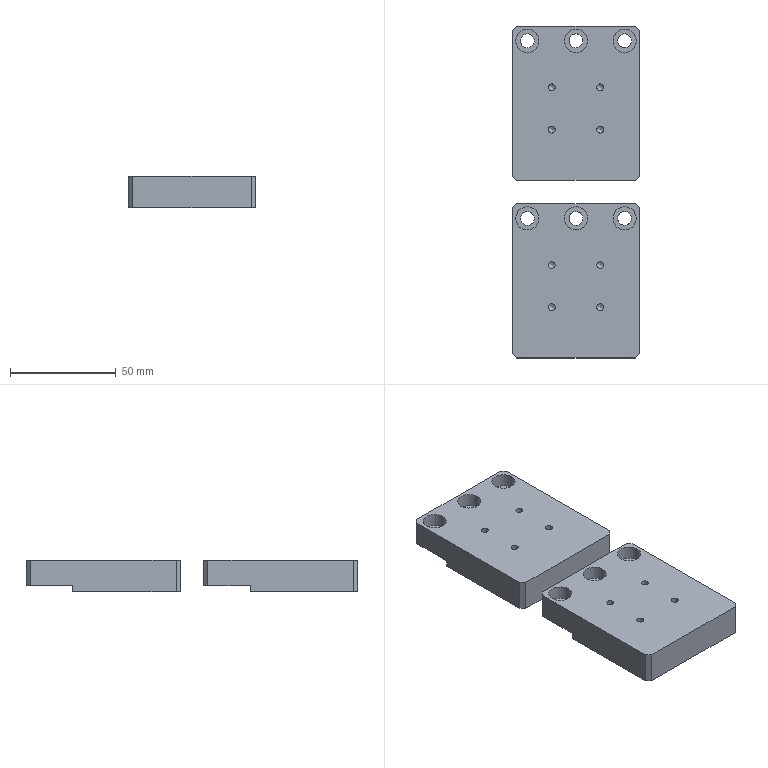CAM job | NX | 3-axis milling, drilling | part box 60 x 157 x 15 mm | stock box 65 x 162 x 20 mm
Tools:
number,name,description,diameter,corner_radius,flute_length,length,flutes
6,D6,平底铣刀-粗,6.0,0.0,25.0,75.0,2
9,D10,平底铣刀-粗,10.0,0.0,35.0,75.0,2
7,D6-J,平底铣刀-精,6.0,0.0,25.0,75.0,2
10,D10-J,平底铣刀-精,10.0,0.0,35.0,75.0,2
1,D80R0.8飞刀,圆鼻刀-粗,80.0,0.8,50.0,75.0,2
1,D80R0.8飞刀-J,圆鼻刀-精,80.0,0.8,50.0,75.0,2
2,D6倒角刀,倒角刀,6.0,0.0,3.0,25.0,2
21,M4X0.7,丝锥,3.3,0.0,35.0,50.0,2
17,ZT6.6,钻头,6.6,0.0,35.0,50.0,2
13,钻头3.3,Twist Drill 3.3 mm,3.3,0.0,35.0,35.008,2
Operations:
program,operation,operation_type,tool,method,geometry_group,spindle_rpm,surface_speed,feed_per_tooth,feed_cut,feed_plunge,cut_length_mm,path_length_mm,cut_time_min,machine_time_min
B,底壁铣飞面一刀开粗_COPY,VolumeBased25DMillingOperation,D80R0.8飞刀,分层开粗-切深K-步距G,W-B,2800.0,703.696,0.5357,3000.0,100.0,2386.746,4674.966,0.7956,1.024
B,底壁铣飞面一刀精光_COPY,VolumeBased25DMillingOperation,D80R0.8飞刀-J,侧刃精光-切深K-步距G,W-B,4000.0,1005.28,0.125,1000.0,100.0,264.998,300.998,0.265,0.2686
B,底壁铣分层开粗-中_COPY,VolumeBased25DMillingOperation,D10,分层开粗-切深K-步距G,W-B,8000.0,251.32,0.25,4000.0,100.0,3038.93,3339.684,0.7597,0.7898
B,铣倒角_2,PlanarMilling,D6倒角刀,METHOD,W-B,8000.0,150.796,0.075,1200.0,100.0,122.676,588.061,0.1022,0.1488
B,C0.3平面去毛刺6X45L__COPY,SurfaceContour,D6倒角刀,爬面_倒角-切深0-步距G,W-B,8000.0,150.796,0.0938,1500.0,90.0,779.275,1448.738,0.5211,0.588
B,底壁铣精光底面-中_COPY,VolumeBased25DMillingOperation,D10-J,精光步距切深关,W-B,8000.0,251.32,0.0625,1000.0,100.0,742.944,931.194,0.7429,0.7618
B,底壁铣精光侧面-中-选底面_COPY,VolumeBased25DMillingOperation,D10-J,侧刃精光-切深K-步距G,W-B,8000.0,251.32,0.0625,1000.0,100.0,157.364,335.31,0.1574,0.1752
A,顶面,FaceMilling,D80R0.8飞刀,侧刃精光-切深K-步距G,W-A,4000.0,1005.31,0.125,1000.0,100.0,534.667,570.667,0.5347,0.5383
A,外形粗_2,VolumeBased25DMillingOperation,D10,METHOD,W-A,8000.0,251.327,0.3125,5000.0,80.0,12324.077,12515.177,2.465,2.484
A,打点-深0.8,Operation,D6倒角刀,NONE,W-A,8000.0,150.796,0.0312,500.0,90.0,25.2,416.7,0.0504,0.0895
A,沉头孔-钻孔0段,Operation,ZT6.6,NONE,W-A,1200.0,24.881,0.0625,150.0,90.0,101.897,424.887,0.6793,0.7116
A,盲锥孔-M4螺纹底孔,Operation,钻头3.3,NONE,W-A,3000.0,31.102,0.02,120.0,90.0,112.0,461.151,0.9333,0.9682
A,铣孔开粗D6_1,CylinderMilling,D6,NONE,W-A,8000.0,150.796,0.075,1200.0,100.0,1384.998,1859.398,1.154,1.202
A,铣孔精光D6_1,CylinderMilling,D6-J,精光步距切深关,W-A,8000.0,150.796,0.0312,500.0,100.0,267.692,745.092,0.5354,0.5831
A,仅选体,SurfaceContour,D6倒角刀,METHOD,W-A,8000.0,150.796,0.1875,3000.0,100.0,557.231,712.334,0.1857,0.2013
A,钻倒角_1,Operation,D6倒角刀,METHOD,W-A,8000.0,150.796,0.0312,500.0,0.0,41.6,335.555,0.0832,0.1126
A,铣倒角_1,PlanarMilling,D6倒角刀,NONE,W-A,8000.0,150.796,0.05,800.0,100.0,260.356,659.679,0.3254,0.3654
A,盲锥孔-攻牙M4,Operation,M4X0.7,METHOD,W-A,800.0,8.294,0.0004,0.7,90.0,88.0,413.151,125.714,125.747
A,外形半精_2,VolumeBased25DMillingOperation,D10-J,METHOD,W-A,8000.0,251.327,0.0625,1000.0,100.0,605.838,675.438,0.6058,0.6128